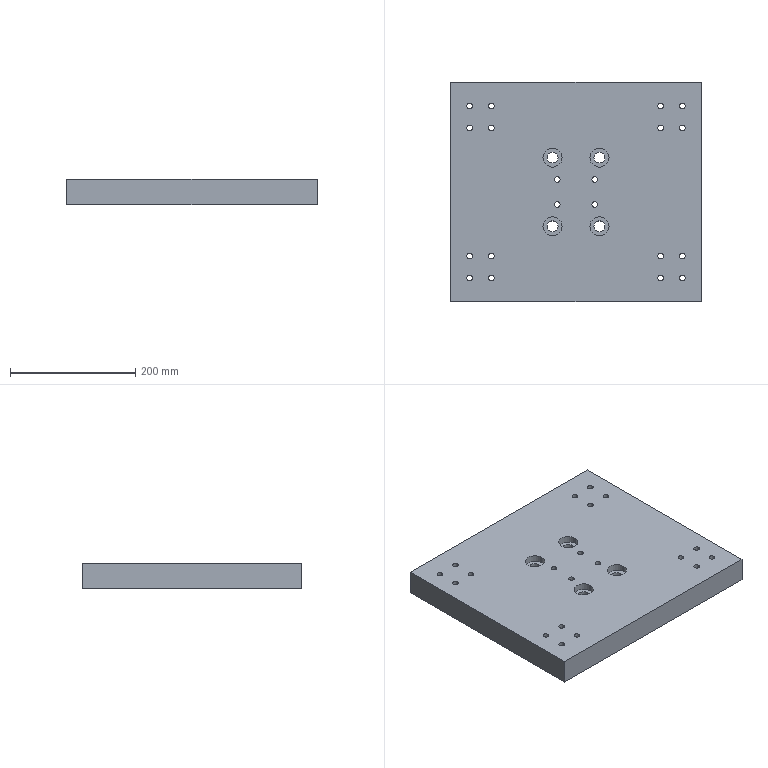Part | SolidWorks | features BaseBody 1 | 1 solid | 126 faces | box 400 x 350 x 40 mm | volume 5471018 mm3 | cylinder 96 | plane 30 | commonest cylinder face diameters 9 x40 15 x40 17.5 x8 30.71 x8